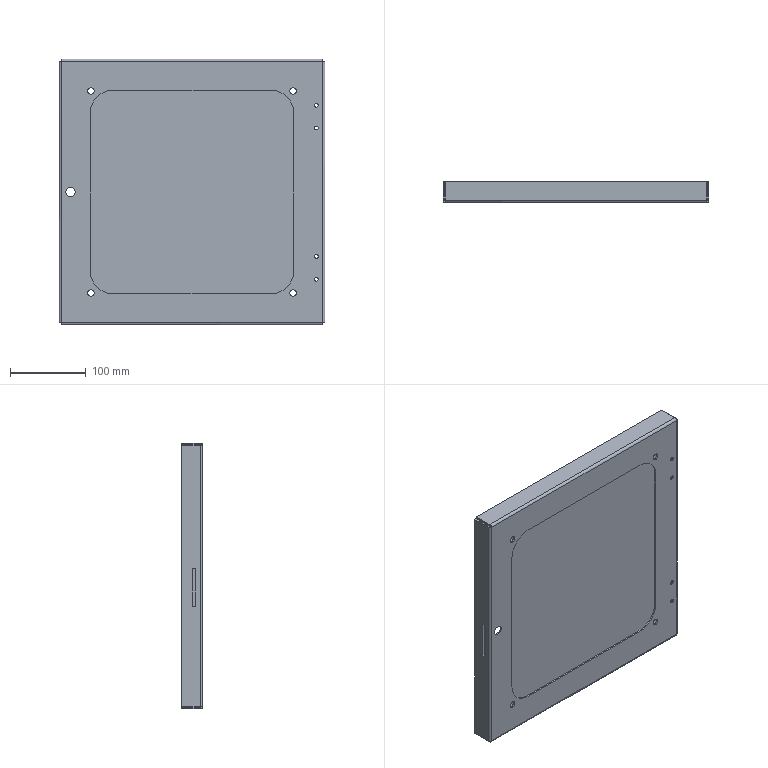Part | SolidWorks | 2 solids | 84 faces | box 350 x 28 x 350 mm | volume 567383 mm3 | cylinder 38 | plane 38 | spline 8 | commonest cylinder face diameters 8.5 x16 5 x8 2 x4 6 x4 60 x4 12.4 x2